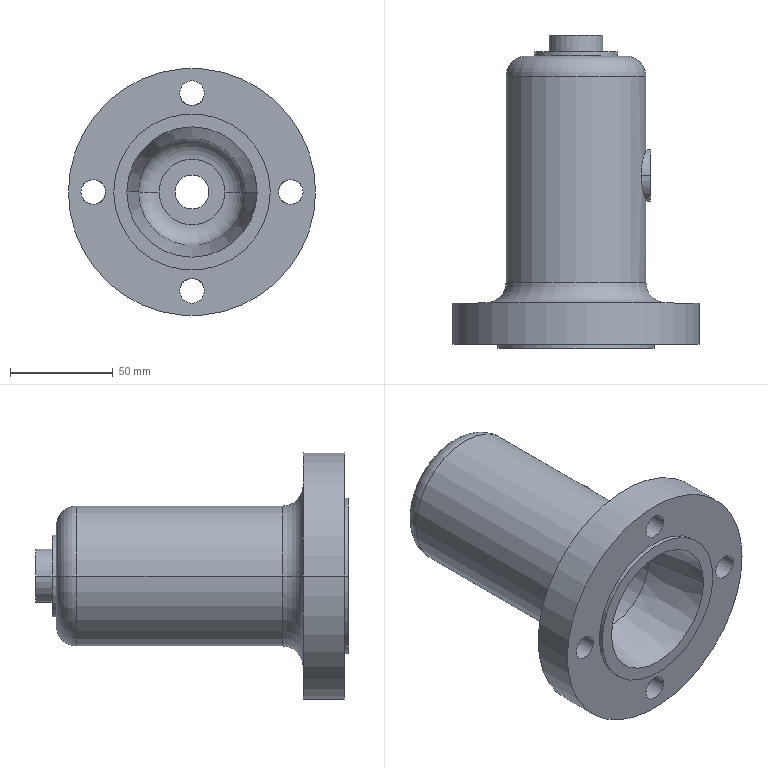Part | SolidWorks | features ICE 3, HoleWzd 1, Revolution 1 | 1 solid | 42 faces | box 120 x 152 x 120 mm | volume 371857 mm3 | cylinder 26 | plane 8 | torus 6 | cone 2 | commonest cylinder face diameters 12 x8 14 x2 16.5 x2 25 x2 26 x2 40 x2